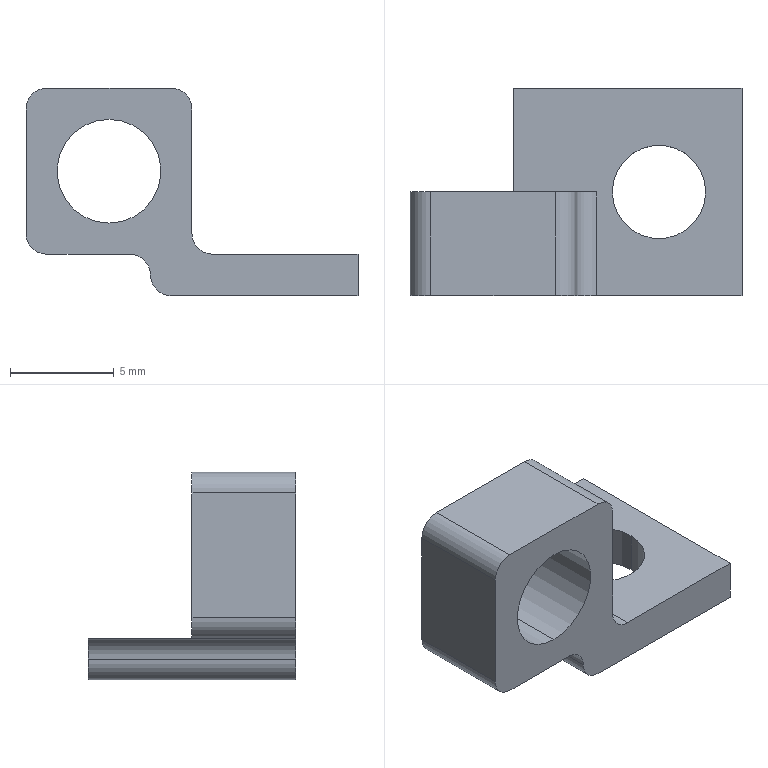Part | SolidWorks | features ICE 4, Fillet 2, Extrusion 1 | 1 solid | 20 faces | box 16 x 10 x 10 mm | volume 387.871 mm3 | cylinder 10 | plane 10 | commonest cylinder face diameters 2 x6 4.5 x2 5 x2
STEP:
#1=CARTESIAN_POINT('',(-8.,0.,3.5));
#2=VERTEX_POINT('',#1);
#3=CARTESIAN_POINT('',(-8.,0.,8.5));
#4=VERTEX_POINT('',#3);
#5=CARTESIAN_POINT('',(-8.,0.,6.));
#6=DIRECTION('',(0.,1.,0.));
#7=DIRECTION('',(0.,0.,-1.));
#8=AXIS2_PLACEMENT_3D('',#5,#6,#7);
#9=CIRCLE('',#8,2.5);
#10=EDGE_CURVE('',#2,#4,#9,.T.);
#11=ORIENTED_EDGE('',*,*,#10,.T.);
#12=CARTESIAN_POINT('',(-8.,-5.,8.5));
#13=VERTEX_POINT('',#12);
#14=CARTESIAN_POINT('',(-8.,5.,8.5));
#15=DIRECTION('',(0.,-1.,0.));
#16=VECTOR('',#15,1000.);
#17=LINE('',#14,#16);
#18=EDGE_CURVE('',#4,#13,#17,.T.);
#19=ORIENTED_EDGE('',*,*,#18,.T.);
#20=CARTESIAN_POINT('',(-8.,-5.,3.5));
#21=VERTEX_POINT('',#20);
#22=CARTESIAN_POINT('',(-8.,-5.,6.));
#23=DIRECTION('',(0.,-1.,0.));
#24=DIRECTION('',(0.,0.,-1.));
#25=AXIS2_PLACEMENT_3D('',#22,#23,#24);
#26=CIRCLE('',#25,2.5);
#27=EDGE_CURVE('',#13,#21,#26,.T.);
#28=ORIENTED_EDGE('',*,*,#27,.T.);
#29=CARTESIAN_POINT('',(-8.,5.,3.5));
#30=DIRECTION('',(0.,-1.,0.));
#31=VECTOR('',#30,1000.);
#32=LINE('',#29,#31);
#33=EDGE_CURVE('',#2,#21,#32,.T.);
#34=ORIENTED_EDGE('',*,*,#33,.F.);
#35=EDGE_LOOP('',(#11,#19,#28,#34));
#36=FACE_OUTER_BOUND('',#35,.T.);
#37=CARTESIAN_POINT('',(-8.,5.,6.));
#38=DIRECTION('',(0.,-1.,0.));
#39=DIRECTION('',(0.,0.,-1.));
#40=AXIS2_PLACEMENT_3D('',#37,#38,#39);
#41=CYLINDRICAL_SURFACE('',#40,2.5);
#42=ADVANCED_FACE('',(#36),#41,.F.);
#43=CARTESIAN_POINT('',(-2.25,0.,2.));
#44=VERTEX_POINT('',#43);
#45=CARTESIAN_POINT('',(2.25,0.,2.));
#46=VERTEX_POINT('',#45);
#47=CARTESIAN_POINT('',(0.,0.,2.));
#48=DIRECTION('',(0.,0.,1.));
#49=DIRECTION('',(1.,0.,0.));
#50=AXIS2_PLACEMENT_3D('',#47,#48,#49);
#51=CIRCLE('',#50,2.25);
#52=EDGE_CURVE('',#44,#46,#51,.T.);
#53=ORIENTED_EDGE('',*,*,#52,.T.);
#54=CARTESIAN_POINT('',(2.25,0.,0.));
#55=VERTEX_POINT('',#54);
#56=CARTESIAN_POINT('',(2.25,0.,2.));
#57=DIRECTION('',(0.,0.,-1.));
#58=VECTOR('',#57,1000.);
#59=LINE('',#56,#58);
#60=EDGE_CURVE('',#46,#55,#59,.T.);
#61=ORIENTED_EDGE('',*,*,#60,.T.);
#62=CARTESIAN_POINT('',(-2.25,0.,0.));
#63=VERTEX_POINT('',#62);
#64=CARTESIAN_POINT('',(0.,0.,0.));
#65=DIRECTION('',(0.,0.,1.));
#66=DIRECTION('',(1.,0.,0.));
#67=AXIS2_PLACEMENT_3D('',#64,#65,#66);
#68=CIRCLE('',#67,2.25);
#69=EDGE_CURVE('',#63,#55,#68,.T.);
#70=ORIENTED_EDGE('',*,*,#69,.F.);
#71=CARTESIAN_POINT('',(-2.25,0.,2.));
#72=DIRECTION('',(0.,0.,-1.));
#73=VECTOR('',#72,1000.);
#74=LINE('',#71,#73);
#75=EDGE_CURVE('',#44,#63,#74,.T.);
#76=ORIENTED_EDGE('',*,*,#75,.F.);
#77=EDGE_LOOP('',(#53,#61,#70,#76));
#78=FACE_OUTER_BOUND('',#77,.T.);
#79=CARTESIAN_POINT('',(0.,0.,2.));
#80=DIRECTION('',(0.,0.,-1.));
#81=DIRECTION('',(-1.,0.,0.));
#82=AXIS2_PLACEMENT_3D('',#79,#80,#81);
#83=CYLINDRICAL_SURFACE('',#82,2.25);
#84=ADVANCED_FACE('',(#78),#83,.F.);
#85=CARTESIAN_POINT('',(4.,5.,2.));
#86=VERTEX_POINT('',#85);
#87=CARTESIAN_POINT('',(-7.,5.,2.));
#88=VERTEX_POINT('',#87);
#89=CARTESIAN_POINT('',(-4.,5.,2.));
#90=DIRECTION('',(-1.,0.,0.));
#91=VECTOR('',#90,1000.);
#92=LINE('',#89,#91);
#93=EDGE_CURVE('',#86,#88,#92,.T.);
#94=ORIENTED_EDGE('',*,*,#93,.T.);
#95=CARTESIAN_POINT('',(-7.,0.,2.));
#96=VERTEX_POINT('',#95);
#97=CARTESIAN_POINT('',(-7.,5.,2.));
#98=DIRECTION('',(0.,-1.,0.));
#99=VECTOR('',#98,1000.);
#100=LINE('',#97,#99);
#101=EDGE_CURVE('',#88,#96,#100,.T.);
#102=ORIENTED_EDGE('',*,*,#101,.T.);
#103=CARTESIAN_POINT('',(-3.,0.,2.));
#104=VERTEX_POINT('',#103);
#105=CARTESIAN_POINT('',(-14.247,0.,2.));
#106=DIRECTION('',(-1.,0.,0.));
#107=VECTOR('',#106,1000.);
#108=LINE('',#105,#107);
#109=EDGE_CURVE('',#104,#96,#108,.T.);
#110=ORIENTED_EDGE('',*,*,#109,.F.);
#111=CARTESIAN_POINT('',(-3.,-5.,2.));
#112=VERTEX_POINT('',#111);
#113=CARTESIAN_POINT('',(-3.,-5.,2.));
#114=DIRECTION('',(0.,-1.,0.));
#115=VECTOR('',#114,1000.);
#116=LINE('',#113,#115);
#117=EDGE_CURVE('',#104,#112,#116,.T.);
#118=ORIENTED_EDGE('',*,*,#117,.T.);
#119=CARTESIAN_POINT('',(4.,-5.,2.));
#120=VERTEX_POINT('',#119);
#121=CARTESIAN_POINT('',(-4.,-5.,2.));
#122=DIRECTION('',(1.,0.,0.));
#123=VECTOR('',#122,1000.);
#124=LINE('',#121,#123);
#125=EDGE_CURVE('',#112,#120,#124,.T.);
#126=ORIENTED_EDGE('',*,*,#125,.T.);
#127=CARTESIAN_POINT('',(4.,5.,2.));
#128=DIRECTION('',(0.,1.,0.));
#129=VECTOR('',#128,1000.);
#130=LINE('',#127,#129);
#131=EDGE_CURVE('',#120,#86,#130,.T.);
#132=ORIENTED_EDGE('',*,*,#131,.T.);
#133=EDGE_LOOP('',(#94,#102,#110,#118,#126,#132));
#134=FACE_OUTER_BOUND('',#133,.T.);
#135=ORIENTED_EDGE('',*,*,#52,.F.);
#136=CARTESIAN_POINT('',(0.,0.,2.));
#137=DIRECTION('',(0.,0.,1.));
#138=DIRECTION('',(1.,0.,0.));
#139=AXIS2_PLACEMENT_3D('',#136,#137,#138);
#140=CIRCLE('',#139,2.25);
#141=EDGE_CURVE('',#46,#44,#140,.T.);
#142=ORIENTED_EDGE('',*,*,#141,.F.);
#143=EDGE_LOOP('',(#135,#142));
#144=FACE_BOUND('',#143,.T.);
#145=CARTESIAN_POINT('',(0.,0.,2.));
#146=DIRECTION('',(0.,0.,1.));
#147=DIRECTION('',(1.,0.,0.));
#148=AXIS2_PLACEMENT_3D('',#145,#146,#147);
#149=PLANE('',#148);
#150=ADVANCED_FACE('',(#134,#144),#149,.T.);
#151=CARTESIAN_POINT('',(-5.,-5.,0.));
#152=VERTEX_POINT('',#151);
#153=CARTESIAN_POINT('',(4.,-5.,0.));
#154=VERTEX_POINT('',#153);
#155=CARTESIAN_POINT('',(-4.,-5.,0.));
#156=DIRECTION('',(1.,0.,0.));
#157=VECTOR('',#156,1000.);
#158=LINE('',#155,#157);
#159=EDGE_CURVE('',#152,#154,#158,.T.);
#160=ORIENTED_EDGE('',*,*,#159,.F.);
#161=CARTESIAN_POINT('',(-5.,5.,0.));
#162=VERTEX_POINT('',#161);
#163=CARTESIAN_POINT('',(-5.,5.,0.));
#164=DIRECTION('',(0.,1.,0.));
#165=VECTOR('',#164,1000.);
#166=LINE('',#163,#165);
#167=EDGE_CURVE('',#152,#162,#166,.T.);
#168=ORIENTED_EDGE('',*,*,#167,.T.);
#169=CARTESIAN_POINT('',(4.,5.,0.));
#170=VERTEX_POINT('',#169);
#171=CARTESIAN_POINT('',(-4.,5.,0.));
#172=DIRECTION('',(-1.,0.,0.));
#173=VECTOR('',#172,1000.);
#174=LINE('',#171,#173);
#175=EDGE_CURVE('',#170,#162,#174,.T.);
#176=ORIENTED_EDGE('',*,*,#175,.F.);
#177=CARTESIAN_POINT('',(4.,5.,0.));
#178=DIRECTION('',(0.,1.,0.));
#179=VECTOR('',#178,1000.);
#180=LINE('',#177,#179);
#181=EDGE_CURVE('',#154,#170,#180,.T.);
#182=ORIENTED_EDGE('',*,*,#181,.F.);
#183=EDGE_LOOP('',(#160,#168,#176,#182));
#184=FACE_OUTER_BOUND('',#183,.T.);
#185=ORIENTED_EDGE('',*,*,#69,.T.);
#186=CARTESIAN_POINT('',(0.,0.,0.));
#187=DIRECTION('',(0.,0.,1.));
#188=DIRECTION('',(1.,0.,0.));
#189=AXIS2_PLACEMENT_3D('',#186,#187,#188);
#190=CIRCLE('',#189,2.25);
#191=EDGE_CURVE('',#55,#63,#190,.T.);
#192=ORIENTED_EDGE('',*,*,#191,.T.);
#193=EDGE_LOOP('',(#185,#192));
#194=FACE_BOUND('',#193,.T.);
#195=CARTESIAN_POINT('',(0.,0.,0.));
#196=DIRECTION('',(0.,0.,1.));
#197=DIRECTION('',(1.,0.,0.));
#198=AXIS2_PLACEMENT_3D('',#195,#196,#197);
#199=PLANE('',#198);
#200=ADVANCED_FACE('',(#184,#194),#199,.F.);
#201=ORIENTED_EDGE('',*,*,#181,.T.);
#202=CARTESIAN_POINT('',(4.,5.,2.));
#203=DIRECTION('',(0.,0.,-1.));
#204=VECTOR('',#203,1000.);
#205=LINE('',#202,#204);
#206=EDGE_CURVE('',#86,#170,#205,.T.);
#207=ORIENTED_EDGE('',*,*,#206,.F.);
#208=ORIENTED_EDGE('',*,*,#131,.F.);
#209=CARTESIAN_POINT('',(4.,-5.,2.));
#210=DIRECTION('',(0.,0.,-1.));
#211=VECTOR('',#210,1000.);
#212=LINE('',#209,#211);
#213=EDGE_CURVE('',#120,#154,#212,.T.);
#214=ORIENTED_EDGE('',*,*,#213,.T.);
#215=EDGE_LOOP('',(#201,#207,#208,#214));
#216=FACE_OUTER_BOUND('',#215,.T.);
#217=CARTESIAN_POINT('',(4.,5.,2.));
#218=DIRECTION('',(-1.,0.,0.));
#219=DIRECTION('',(0.,-1.,0.));
#220=AXIS2_PLACEMENT_3D('',#217,#218,#219);
#221=PLANE('',#220);
#222=ADVANCED_FACE('',(#216),#221,.F.);
#223=CARTESIAN_POINT('',(-6.,5.,1.));
#224=VERTEX_POINT('',#223);
#225=CARTESIAN_POINT('',(-7.,5.,1.));
#226=DIRECTION('',(0.,-1.,0.));
#227=DIRECTION('',(0.,0.,-1.));
#228=AXIS2_PLACEMENT_3D('',#225,#226,#227);
#229=CIRCLE('',#228,1.);
#230=EDGE_CURVE('',#224,#88,#229,.T.);
#231=ORIENTED_EDGE('',*,*,#230,.T.);
#232=ORIENTED_EDGE('',*,*,#93,.F.);
#233=ORIENTED_EDGE('',*,*,#206,.T.);
#234=ORIENTED_EDGE('',*,*,#175,.T.);
#235=CARTESIAN_POINT('',(-5.,5.,1.));
#236=DIRECTION('',(0.,1.,0.));
#237=DIRECTION('',(0.,0.,-1.));
#238=AXIS2_PLACEMENT_3D('',#235,#236,#237);
#239=CIRCLE('',#238,1.);
#240=EDGE_CURVE('',#162,#224,#239,.T.);
#241=ORIENTED_EDGE('',*,*,#240,.T.);
#242=EDGE_LOOP('',(#231,#232,#233,#234,#241));
#243=FACE_OUTER_BOUND('',#242,.T.);
#244=CARTESIAN_POINT('',(-4.,5.,2.));
#245=DIRECTION('',(0.,-1.,0.));
#246=DIRECTION('',(0.,0.,-1.));
#247=AXIS2_PLACEMENT_3D('',#244,#245,#246);
#248=PLANE('',#247);
#249=ADVANCED_FACE('',(#243),#248,.F.);
#250=CARTESIAN_POINT('',(-8.,-5.,6.));
#251=DIRECTION('',(0.,-1.,0.));
#252=DIRECTION('',(0.,0.,-1.));
#253=AXIS2_PLACEMENT_3D('',#250,#251,#252);
#254=CIRCLE('',#253,2.5);
#255=EDGE_CURVE('',#21,#13,#254,.T.);
#256=ORIENTED_EDGE('',*,*,#255,.F.);
#257=ORIENTED_EDGE('',*,*,#27,.F.);
#258=EDGE_LOOP('',(#256,#257));
#259=FACE_BOUND('',#258,.T.);
#260=CARTESIAN_POINT('',(-7.,-5.,2.));
#261=VERTEX_POINT('',#260);
#262=CARTESIAN_POINT('',(-6.,-5.,1.));
#263=VERTEX_POINT('',#262);
#264=CARTESIAN_POINT('',(-7.,-5.,1.));
#265=DIRECTION('',(0.,1.,0.));
#266=DIRECTION('',(0.,0.,1.));
#267=AXIS2_PLACEMENT_3D('',#264,#265,#266);
#268=CIRCLE('',#267,1.);
#269=EDGE_CURVE('',#261,#263,#268,.T.);
#270=ORIENTED_EDGE('',*,*,#269,.T.);
#271=CARTESIAN_POINT('',(-5.,-5.,1.));
#272=DIRECTION('',(0.,-1.,0.));
#273=DIRECTION('',(0.,0.,1.));
#274=AXIS2_PLACEMENT_3D('',#271,#272,#273);
#275=CIRCLE('',#274,1.);
#276=EDGE_CURVE('',#263,#152,#275,.T.);
#277=ORIENTED_EDGE('',*,*,#276,.T.);
#278=ORIENTED_EDGE('',*,*,#159,.T.);
#279=ORIENTED_EDGE('',*,*,#213,.F.);
#280=ORIENTED_EDGE('',*,*,#125,.F.);
#281=CARTESIAN_POINT('',(-4.,-5.,3.));
#282=VERTEX_POINT('',#281);
#283=CARTESIAN_POINT('',(-3.,-5.,3.));
#284=DIRECTION('',(0.,1.,0.));
#285=DIRECTION('',(0.,0.,1.));
#286=AXIS2_PLACEMENT_3D('',#283,#284,#285);
#287=CIRCLE('',#286,1.);
#288=EDGE_CURVE('',#112,#282,#287,.T.);
#289=ORIENTED_EDGE('',*,*,#288,.T.);
#290=CARTESIAN_POINT('',(-4.,-5.,9.));
#291=VERTEX_POINT('',#290);
#292=CARTESIAN_POINT('',(-4.,-5.,10.));
#293=DIRECTION('',(0.,0.,-1.));
#294=VECTOR('',#293,1000.);
#295=LINE('',#292,#294);
#296=EDGE_CURVE('',#291,#282,#295,.T.);
#297=ORIENTED_EDGE('',*,*,#296,.F.);
#298=CARTESIAN_POINT('',(-5.,-5.,10.));
#299=VERTEX_POINT('',#298);
#300=CARTESIAN_POINT('',(-5.,-5.,9.));
#301=DIRECTION('',(0.,-1.,0.));
#302=DIRECTION('',(0.,0.,1.));
#303=AXIS2_PLACEMENT_3D('',#300,#301,#302);
#304=CIRCLE('',#303,1.);
#305=EDGE_CURVE('',#291,#299,#304,.T.);
#306=ORIENTED_EDGE('',*,*,#305,.T.);
#307=CARTESIAN_POINT('',(-11.,-5.,10.));
#308=VERTEX_POINT('',#307);
#309=CARTESIAN_POINT('',(-6.,-5.,10.));
#310=DIRECTION('',(-1.,0.,0.));
#311=VECTOR('',#310,1000.);
#312=LINE('',#309,#311);
#313=EDGE_CURVE('',#299,#308,#312,.T.);
#314=ORIENTED_EDGE('',*,*,#313,.T.);
#315=CARTESIAN_POINT('',(-12.,-5.,9.));
#316=VERTEX_POINT('',#315);
#317=CARTESIAN_POINT('',(-11.,-5.,9.));
#318=DIRECTION('',(0.,-1.,0.));
#319=DIRECTION('',(0.,0.,1.));
#320=AXIS2_PLACEMENT_3D('',#317,#318,#319);
#321=CIRCLE('',#320,1.);
#322=EDGE_CURVE('',#308,#316,#321,.T.);
#323=ORIENTED_EDGE('',*,*,#322,.T.);
#324=CARTESIAN_POINT('',(-12.,-5.,3.));
#325=VERTEX_POINT('',#324);
#326=CARTESIAN_POINT('',(-12.,-5.,2.));
#327=DIRECTION('',(0.,0.,1.));
#328=VECTOR('',#327,1000.);
#329=LINE('',#326,#328);
#330=EDGE_CURVE('',#325,#316,#329,.T.);
#331=ORIENTED_EDGE('',*,*,#330,.F.);
#332=CARTESIAN_POINT('',(-11.,-5.,2.));
#333=VERTEX_POINT('',#332);
#334=CARTESIAN_POINT('',(-11.,-5.,3.));
#335=DIRECTION('',(0.,-1.,0.));
#336=DIRECTION('',(0.,0.,1.));
#337=AXIS2_PLACEMENT_3D('',#334,#335,#336);
#338=CIRCLE('',#337,1.);
#339=EDGE_CURVE('',#325,#333,#338,.T.);
#340=ORIENTED_EDGE('',*,*,#339,.T.);
#341=CARTESIAN_POINT('',(-12.,-5.,2.));
#342=DIRECTION('',(1.,0.,0.));
#343=VECTOR('',#342,1000.);
#344=LINE('',#341,#343);
#345=EDGE_CURVE('',#333,#261,#344,.T.);
#346=ORIENTED_EDGE('',*,*,#345,.T.);
#347=EDGE_LOOP('',(#270,#277,#278,#279,#280,#289,#297,#306,#314,#323,#331,#340,#346));
#348=FACE_OUTER_BOUND('',#347,.T.);
#349=CARTESIAN_POINT('',(-4.,-5.,2.));
#350=DIRECTION('',(0.,1.,0.));
#351=DIRECTION('',(0.,0.,1.));
#352=AXIS2_PLACEMENT_3D('',#349,#350,#351);
#353=PLANE('',#352);
#354=ADVANCED_FACE('',(#259,#348),#353,.F.);
#355=ORIENTED_EDGE('',*,*,#60,.F.);
#356=ORIENTED_EDGE('',*,*,#141,.T.);
#357=ORIENTED_EDGE('',*,*,#75,.T.);
#358=ORIENTED_EDGE('',*,*,#191,.F.);
#359=EDGE_LOOP('',(#355,#356,#357,#358));
#360=FACE_OUTER_BOUND('',#359,.T.);
#361=CARTESIAN_POINT('',(0.,0.,2.));
#362=DIRECTION('',(0.,0.,-1.));
#363=DIRECTION('',(-1.,0.,0.));
#364=AXIS2_PLACEMENT_3D('',#361,#362,#363);
#365=CYLINDRICAL_SURFACE('',#364,2.25);
#366=ADVANCED_FACE('',(#360),#365,.F.);
#367=CARTESIAN_POINT('',(-4.,0.,9.));
#368=VERTEX_POINT('',#367);
#369=CARTESIAN_POINT('',(-4.,0.,3.));
#370=VERTEX_POINT('',#369);
#371=CARTESIAN_POINT('',(-4.,0.,10.));
#372=DIRECTION('',(0.,0.,-1.));
#373=VECTOR('',#372,1000.);
#374=LINE('',#371,#373);
#375=EDGE_CURVE('',#368,#370,#374,.T.);
#376=ORIENTED_EDGE('',*,*,#375,.F.);
#377=CARTESIAN_POINT('',(-4.,-5.,9.));
#378=DIRECTION('',(0.,-1.,0.));
#379=VECTOR('',#378,1000.);
#380=LINE('',#377,#379);
#381=EDGE_CURVE('',#368,#291,#380,.T.);
#382=ORIENTED_EDGE('',*,*,#381,.T.);
#383=ORIENTED_EDGE('',*,*,#296,.T.);
#384=CARTESIAN_POINT('',(-4.,5.,3.));
#385=DIRECTION('',(0.,1.,0.));
#386=VECTOR('',#385,1000.);
#387=LINE('',#384,#386);
#388=EDGE_CURVE('',#282,#370,#387,.T.);
#389=ORIENTED_EDGE('',*,*,#388,.T.);
#390=EDGE_LOOP('',(#376,#382,#383,#389));
#391=FACE_OUTER_BOUND('',#390,.T.);
#392=CARTESIAN_POINT('',(-4.,-5.,10.));
#393=DIRECTION('',(1.,0.,0.));
#394=DIRECTION('',(0.,0.,-1.));
#395=AXIS2_PLACEMENT_3D('',#392,#393,#394);
#396=PLANE('',#395);
#397=ADVANCED_FACE('',(#391),#396,.T.);
#398=CARTESIAN_POINT('',(-5.,0.,10.));
#399=VERTEX_POINT('',#398);
#400=CARTESIAN_POINT('',(-5.,5.,10.));
#401=DIRECTION('',(0.,1.,0.));
#402=VECTOR('',#401,1000.);
#403=LINE('',#400,#402);
#404=EDGE_CURVE('',#299,#399,#403,.T.);
#405=ORIENTED_EDGE('',*,*,#404,.T.);
#406=CARTESIAN_POINT('',(-11.,0.,10.));
#407=VERTEX_POINT('',#406);
#408=CARTESIAN_POINT('',(0.,0.,10.));
#409=DIRECTION('',(-1.,0.,0.));
#410=VECTOR('',#409,1000.);
#411=LINE('',#408,#410);
#412=EDGE_CURVE('',#399,#407,#411,.T.);
#413=ORIENTED_EDGE('',*,*,#412,.T.);
#414=CARTESIAN_POINT('',(-11.,-5.,10.));
#415=DIRECTION('',(0.,-1.,0.));
#416=VECTOR('',#415,1000.);
#417=LINE('',#414,#416);
#418=EDGE_CURVE('',#407,#308,#417,.T.);
#419=ORIENTED_EDGE('',*,*,#418,.T.);
#420=ORIENTED_EDGE('',*,*,#313,.F.);
#421=EDGE_LOOP('',(#405,#413,#419,#420));
#422=FACE_OUTER_BOUND('',#421,.T.);
#423=CARTESIAN_POINT('',(0.,0.,10.));
#424=DIRECTION('',(0.,0.,-1.));
#425=DIRECTION('',(-1.,0.,0.));
#426=AXIS2_PLACEMENT_3D('',#423,#424,#425);
#427=PLANE('',#426);
#428=ADVANCED_FACE('',(#422),#427,.F.);
#429=CARTESIAN_POINT('',(-11.,0.,2.));
#430=VERTEX_POINT('',#429);
#431=CARTESIAN_POINT('',(-11.,5.,2.));
#432=DIRECTION('',(0.,1.,0.));
#433=VECTOR('',#432,1000.);
#434=LINE('',#431,#433);
#435=EDGE_CURVE('',#333,#430,#434,.T.);
#436=ORIENTED_EDGE('',*,*,#435,.T.);
#437=CARTESIAN_POINT('',(-14.247,0.,2.));
#438=DIRECTION('',(-1.,0.,0.));
#439=VECTOR('',#438,1000.);
#440=LINE('',#437,#439);
#441=EDGE_CURVE('',#96,#430,#440,.T.);
#442=ORIENTED_EDGE('',*,*,#441,.F.);
#443=CARTESIAN_POINT('',(-7.,5.,2.));
#444=DIRECTION('',(0.,-1.,0.));
#445=VECTOR('',#444,1000.);
#446=LINE('',#443,#445);
#447=EDGE_CURVE('',#96,#261,#446,.T.);
#448=ORIENTED_EDGE('',*,*,#447,.T.);
#449=ORIENTED_EDGE('',*,*,#345,.F.);
#450=EDGE_LOOP('',(#436,#442,#448,#449));
#451=FACE_OUTER_BOUND('',#450,.T.);
#452=CARTESIAN_POINT('',(-12.,5.,2.));
#453=DIRECTION('',(0.,0.,1.));
#454=DIRECTION('',(0.,-1.,0.));
#455=AXIS2_PLACEMENT_3D('',#452,#453,#454);
#456=PLANE('',#455);
#457=ADVANCED_FACE('',(#451),#456,.F.);
#458=CARTESIAN_POINT('',(-12.,0.,3.));
#459=VERTEX_POINT('',#458);
#460=CARTESIAN_POINT('',(-12.,0.,9.));
#461=VERTEX_POINT('',#460);
#462=CARTESIAN_POINT('',(-12.,0.,0.));
#463=DIRECTION('',(0.,0.,1.));
#464=VECTOR('',#463,1000.);
#465=LINE('',#462,#464);
#466=EDGE_CURVE('',#459,#461,#465,.T.);
#467=ORIENTED_EDGE('',*,*,#466,.F.);
#468=CARTESIAN_POINT('',(-12.,-5.,3.));
#469=DIRECTION('',(0.,-1.,0.));
#470=VECTOR('',#469,1000.);
#471=LINE('',#468,#470);
#472=EDGE_CURVE('',#459,#325,#471,.T.);
#473=ORIENTED_EDGE('',*,*,#472,.T.);
#474=ORIENTED_EDGE('',*,*,#330,.T.);
#475=CARTESIAN_POINT('',(-12.,5.,9.));
#476=DIRECTION('',(0.,1.,0.));
#477=VECTOR('',#476,1000.);
#478=LINE('',#475,#477);
#479=EDGE_CURVE('',#316,#461,#478,.T.);
#480=ORIENTED_EDGE('',*,*,#479,.T.);
#481=EDGE_LOOP('',(#467,#473,#474,#480));
#482=FACE_OUTER_BOUND('',#481,.T.);
#483=CARTESIAN_POINT('',(-12.,0.,0.));
#484=DIRECTION('',(-1.,0.,0.));
#485=DIRECTION('',(0.,0.,1.));
#486=AXIS2_PLACEMENT_3D('',#483,#484,#485);
#487=PLANE('',#486);
#488=ADVANCED_FACE('',(#482),#487,.T.);
#489=ORIENTED_EDGE('',*,*,#18,.F.);
#490=CARTESIAN_POINT('',(-8.,0.,6.));
#491=DIRECTION('',(0.,1.,0.));
#492=DIRECTION('',(0.,0.,-1.));
#493=AXIS2_PLACEMENT_3D('',#490,#491,#492);
#494=CIRCLE('',#493,2.5);
#495=EDGE_CURVE('',#4,#2,#494,.T.);
#496=ORIENTED_EDGE('',*,*,#495,.T.);
#497=ORIENTED_EDGE('',*,*,#33,.T.);
#498=ORIENTED_EDGE('',*,*,#255,.T.);
#499=EDGE_LOOP('',(#489,#496,#497,#498));
#500=FACE_OUTER_BOUND('',#499,.T.);
#501=CARTESIAN_POINT('',(-8.,5.,6.));
#502=DIRECTION('',(0.,-1.,0.));
#503=DIRECTION('',(0.,0.,-1.));
#504=AXIS2_PLACEMENT_3D('',#501,#502,#503);
#505=CYLINDRICAL_SURFACE('',#504,2.5);
#506=ADVANCED_FACE('',(#500),#505,.F.);
#507=ORIENTED_EDGE('',*,*,#117,.F.);
#508=CARTESIAN_POINT('',(-3.,0.,3.));
#509=DIRECTION('',(0.,1.,0.));
#510=DIRECTION('',(0.,0.,-1.));
#511=AXIS2_PLACEMENT_3D('',#508,#509,#510);
#512=CIRCLE('',#511,1.);
#513=EDGE_CURVE('',#104,#370,#512,.T.);
#514=ORIENTED_EDGE('',*,*,#513,.T.);
#515=ORIENTED_EDGE('',*,*,#388,.F.);
#516=ORIENTED_EDGE('',*,*,#288,.F.);
#517=EDGE_LOOP('',(#507,#514,#515,#516));
#518=FACE_OUTER_BOUND('',#517,.T.);
#519=CARTESIAN_POINT('',(-3.,0.,3.));
#520=DIRECTION('',(0.,1.,0.));
#521=DIRECTION('',(0.,0.,1.));
#522=AXIS2_PLACEMENT_3D('',#519,#520,#521);
#523=CYLINDRICAL_SURFACE('',#522,1.);
#524=ADVANCED_FACE('',(#518),#523,.F.);
#525=CARTESIAN_POINT('',(-5.,0.,9.));
#526=DIRECTION('',(0.,1.,0.));
#527=DIRECTION('',(0.,0.,-1.));
#528=AXIS2_PLACEMENT_3D('',#525,#526,#527);
#529=CIRCLE('',#528,1.);
#530=EDGE_CURVE('',#399,#368,#529,.T.);
#531=ORIENTED_EDGE('',*,*,#530,.F.);
#532=ORIENTED_EDGE('',*,*,#404,.F.);
#533=ORIENTED_EDGE('',*,*,#305,.F.);
#534=ORIENTED_EDGE('',*,*,#381,.F.);
#535=EDGE_LOOP('',(#531,#532,#533,#534));
#536=FACE_OUTER_BOUND('',#535,.T.);
#537=CARTESIAN_POINT('',(-5.,-5.,9.));
#538=DIRECTION('',(0.,1.,0.));
#539=DIRECTION('',(0.,0.,1.));
#540=AXIS2_PLACEMENT_3D('',#537,#538,#539);
#541=CYLINDRICAL_SURFACE('',#540,1.);
#542=ADVANCED_FACE('',(#536),#541,.T.);
#543=CARTESIAN_POINT('',(-11.,0.,9.));
#544=DIRECTION('',(0.,1.,0.));
#545=DIRECTION('',(0.,0.,-1.));
#546=AXIS2_PLACEMENT_3D('',#543,#544,#545);
#547=CIRCLE('',#546,1.);
#548=EDGE_CURVE('',#461,#407,#547,.T.);
#549=ORIENTED_EDGE('',*,*,#548,.F.);
#550=ORIENTED_EDGE('',*,*,#479,.F.);
#551=ORIENTED_EDGE('',*,*,#322,.F.);
#552=ORIENTED_EDGE('',*,*,#418,.F.);
#553=EDGE_LOOP('',(#549,#550,#551,#552));
#554=FACE_OUTER_BOUND('',#553,.T.);
#555=CARTESIAN_POINT('',(-11.,0.,9.));
#556=DIRECTION('',(0.,-1.,0.));
#557=DIRECTION('',(0.,0.,-1.));
#558=AXIS2_PLACEMENT_3D('',#555,#556,#557);
#559=CYLINDRICAL_SURFACE('',#558,1.);
#560=ADVANCED_FACE('',(#554),#559,.T.);
#561=CARTESIAN_POINT('',(-11.,0.,3.));
#562=DIRECTION('',(0.,1.,0.));
#563=DIRECTION('',(0.,0.,-1.));
#564=AXIS2_PLACEMENT_3D('',#561,#562,#563);
#565=CIRCLE('',#564,1.);
#566=EDGE_CURVE('',#430,#459,#565,.T.);
#567=ORIENTED_EDGE('',*,*,#566,.F.);
#568=ORIENTED_EDGE('',*,*,#435,.F.);
#569=ORIENTED_EDGE('',*,*,#339,.F.);
#570=ORIENTED_EDGE('',*,*,#472,.F.);
#571=EDGE_LOOP('',(#567,#568,#569,#570));
#572=FACE_OUTER_BOUND('',#571,.T.);
#573=CARTESIAN_POINT('',(-11.,0.,3.));
#574=DIRECTION('',(0.,1.,0.));
#575=DIRECTION('',(0.,0.,1.));
#576=AXIS2_PLACEMENT_3D('',#573,#574,#575);
#577=CYLINDRICAL_SURFACE('',#576,1.);
#578=ADVANCED_FACE('',(#572),#577,.T.);
#579=ORIENTED_EDGE('',*,*,#230,.F.);
#580=CARTESIAN_POINT('',(-6.,-5.,1.));
#581=DIRECTION('',(0.,1.,0.));
#582=VECTOR('',#581,1000.);
#583=LINE('',#580,#582);
#584=EDGE_CURVE('',#263,#224,#583,.T.);
#585=ORIENTED_EDGE('',*,*,#584,.F.);
#586=ORIENTED_EDGE('',*,*,#269,.F.);
#587=ORIENTED_EDGE('',*,*,#447,.F.);
#588=ORIENTED_EDGE('',*,*,#101,.F.);
#589=EDGE_LOOP('',(#579,#585,#586,#587,#588));
#590=FACE_OUTER_BOUND('',#589,.T.);
#591=CARTESIAN_POINT('',(-7.,5.,1.));
#592=DIRECTION('',(0.,-1.,0.));
#593=DIRECTION('',(0.,0.,-1.));
#594=AXIS2_PLACEMENT_3D('',#591,#592,#593);
#595=CYLINDRICAL_SURFACE('',#594,1.);
#596=ADVANCED_FACE('',(#590),#595,.F.);
#597=ORIENTED_EDGE('',*,*,#276,.F.);
#598=ORIENTED_EDGE('',*,*,#584,.T.);
#599=ORIENTED_EDGE('',*,*,#240,.F.);
#600=ORIENTED_EDGE('',*,*,#167,.F.);
#601=EDGE_LOOP('',(#597,#598,#599,#600));
#602=FACE_OUTER_BOUND('',#601,.T.);
#603=CARTESIAN_POINT('',(-5.,0.,1.));
#604=DIRECTION('',(0.,-1.,0.));
#605=DIRECTION('',(0.,0.,-1.));
#606=AXIS2_PLACEMENT_3D('',#603,#604,#605);
#607=CYLINDRICAL_SURFACE('',#606,1.);
#608=ADVANCED_FACE('',(#602),#607,.T.);
#609=ORIENTED_EDGE('',*,*,#109,.T.);
#610=ORIENTED_EDGE('',*,*,#441,.T.);
#611=ORIENTED_EDGE('',*,*,#566,.T.);
#612=ORIENTED_EDGE('',*,*,#466,.T.);
#613=ORIENTED_EDGE('',*,*,#548,.T.);
#614=ORIENTED_EDGE('',*,*,#412,.F.);
#615=ORIENTED_EDGE('',*,*,#530,.T.);
#616=ORIENTED_EDGE('',*,*,#375,.T.);
#617=ORIENTED_EDGE('',*,*,#513,.F.);
#618=EDGE_LOOP('',(#609,#610,#611,#612,#613,#614,#615,#616,#617));
#619=FACE_OUTER_BOUND('',#618,.T.);
#620=ORIENTED_EDGE('',*,*,#10,.F.);
#621=ORIENTED_EDGE('',*,*,#495,.F.);
#622=EDGE_LOOP('',(#620,#621));
#623=FACE_BOUND('',#622,.T.);
#624=CARTESIAN_POINT('',(0.,0.,0.));
#625=DIRECTION('',(0.,-1.,0.));
#626=DIRECTION('',(0.,0.,-1.));
#627=AXIS2_PLACEMENT_3D('',#624,#625,#626);
#628=PLANE('',#627);
#629=ADVANCED_FACE('',(#619,#623),#628,.F.);
#630=CLOSED_SHELL('',(#42,#84,#150,#200,#222,#249,#354,#366,#397,#428,#457,#488,#506,#524,#542,#560,#578,#596,#608,#629));
#631=MANIFOLD_SOLID_BREP('',#630);
#632=CARTESIAN_POINT('',(0.,0.,0.));
#633=DIRECTION('',(0.,0.,1.));
#634=DIRECTION('',(1.,0.,0.));
#635=AXIS2_PLACEMENT_3D('',#632,#633,#634);
#636=(LENGTH_UNIT()NAMED_UNIT(*)SI_UNIT(.MILLI.,.METRE.));
#637=UNCERTAINTY_MEASURE_WITH_UNIT(LENGTH_MEASURE(0.00001),#636,'','');
#638=(NAMED_UNIT(*)PLANE_ANGLE_UNIT()SI_UNIT($,.RADIAN.));
#639=(NAMED_UNIT(*)SI_UNIT($,.STERADIAN.)SOLID_ANGLE_UNIT());
#640=(GEOMETRIC_REPRESENTATION_CONTEXT(3)GLOBAL_UNCERTAINTY_ASSIGNED_CONTEXT((#637))GLOBAL_UNIT_ASSIGNED_CONTEXT((#636,#638,#639))REPRESENTATION_CONTEXT('',''));
#641=ADVANCED_BREP_SHAPE_REPRESENTATION('',(#631,#635),#640);